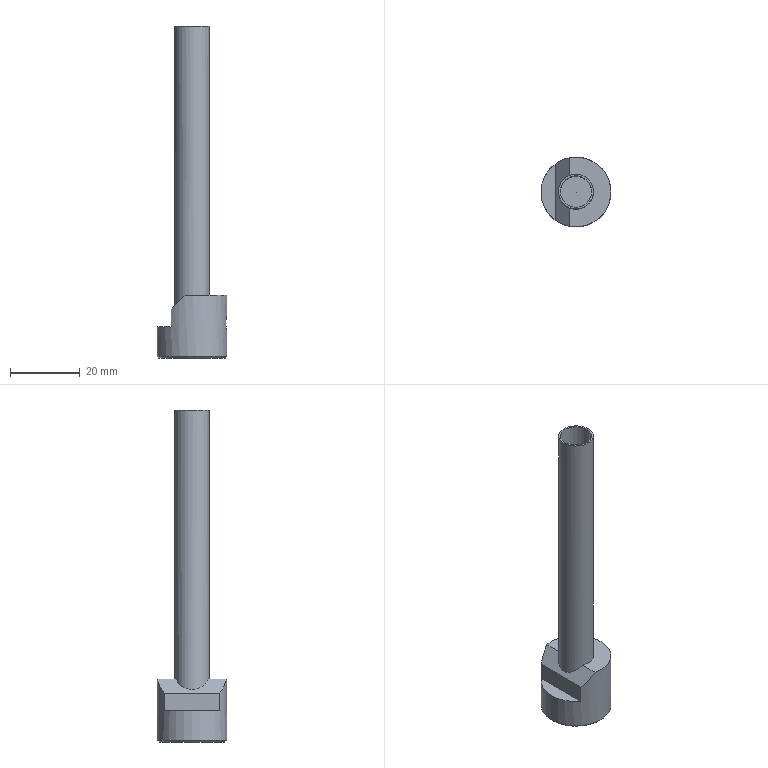Part | STEP file | SL2-MOLD_id178_xmt_txt | 1 solid | 15 faces | box 20 x 20 x 95 mm | volume 5358 mm3 | plane 7 | cylinder 5 | cone 3 | commonest cylinder face diameters 3.3 x1 5 x1 9 x1 10 x1 20 x1
STEP:
#1=CARTESIAN_POINT('',(43.,-50.,-35.));
#2=VERTEX_POINT('',#1);
#3=CARTESIAN_POINT('',(43.,-50.,-40.));
#4=VERTEX_POINT('',#3);
#5=CARTESIAN_POINT('',(43.,-50.,-37.5));
#6=DIRECTION('',(0.,0.,-1.));
#7=VECTOR('',#6,1.);
#8=LINE('',#5,#7);
#9=EDGE_CURVE('',#2,#4,#8,.T.);
#10=ORIENTED_EDGE('',*,*,#9,.F.);
#11=CARTESIAN_POINT('',(43.,-34.,-35.));
#12=VERTEX_POINT('',#11);
#13=CARTESIAN_POINT('',(43.,-42.,-35.));
#14=DIRECTION('',(0.,1.,0.));
#15=VECTOR('',#14,1.);
#16=LINE('',#13,#15);
#17=EDGE_CURVE('',#2,#12,#16,.T.);
#18=ORIENTED_EDGE('',*,*,#17,.T.);
#19=CARTESIAN_POINT('',(43.,-34.,-40.));
#20=VERTEX_POINT('',#19);
#21=CARTESIAN_POINT('',(43.,-34.,-37.5));
#22=DIRECTION('',(0.,0.,1.));
#23=VECTOR('',#22,1.);
#24=LINE('',#21,#23);
#25=EDGE_CURVE('',#20,#12,#24,.T.);
#26=ORIENTED_EDGE('',*,*,#25,.F.);
#27=CARTESIAN_POINT('',(43.,-42.,-40.));
#28=DIRECTION('',(0.,1.,0.));
#29=VECTOR('',#28,1.);
#30=LINE('',#27,#29);
#31=EDGE_CURVE('',#4,#20,#30,.T.);
#32=ORIENTED_EDGE('',*,*,#31,.F.);
#33=EDGE_LOOP('',(#10,#18,#26,#32));
#34=FACE_OUTER_BOUND('',#33,.T.);
#35=CARTESIAN_POINT('',(43.,-42.,-46.));
#36=DIRECTION('',(-1.,0.,0.));
#37=DIRECTION('',(0.,0.,1.));
#38=AXIS2_PLACEMENT_3D('',#35,#36,#37);
#39=PLANE('',#38);
#40=ADVANCED_FACE('',(#34),#39,.T.);
#41=CARTESIAN_POINT('',(47.,-51.798,-31.));
#42=VERTEX_POINT('',#41);
#43=CARTESIAN_POINT('',(47.,-32.202,-31.));
#44=VERTEX_POINT('',#43);
#45=CARTESIAN_POINT('',(49.,-42.,-31.));
#46=DIRECTION('',(0.,0.,1.));
#47=DIRECTION('',(-1.,0.,0.));
#48=AXIS2_PLACEMENT_3D('',#45,#46,#47);
#49=CIRCLE('',#48,10.);
#50=EDGE_CURVE('',#42,#44,#49,.T.);
#51=ORIENTED_EDGE('',*,*,#50,.T.);
#52=CARTESIAN_POINT('',(47.,-37.417,-31.));
#53=VERTEX_POINT('',#52);
#54=CARTESIAN_POINT('',(47.,-42.,-31.));
#55=DIRECTION('',(0.,-1.,0.));
#56=VECTOR('',#55,1.);
#57=LINE('',#54,#56);
#58=EDGE_CURVE('',#44,#53,#57,.T.);
#59=ORIENTED_EDGE('',*,*,#58,.T.);
#60=CARTESIAN_POINT('',(47.,-46.583,-31.));
#61=VERTEX_POINT('',#60);
#62=CARTESIAN_POINT('',(49.,-42.,-31.));
#63=DIRECTION('',(0.,0.,-1.));
#64=DIRECTION('',(-1.,0.,0.));
#65=AXIS2_PLACEMENT_3D('',#62,#63,#64);
#66=CIRCLE('',#65,5.);
#67=EDGE_CURVE('',#53,#61,#66,.T.);
#68=ORIENTED_EDGE('',*,*,#67,.T.);
#69=CARTESIAN_POINT('',(47.,-42.,-31.));
#70=DIRECTION('',(0.,-1.,0.));
#71=VECTOR('',#70,1.);
#72=LINE('',#69,#71);
#73=EDGE_CURVE('',#61,#42,#72,.T.);
#74=ORIENTED_EDGE('',*,*,#73,.T.);
#75=EDGE_LOOP('',(#51,#59,#68,#74));
#76=FACE_OUTER_BOUND('',#75,.T.);
#77=CARTESIAN_POINT('',(49.,-42.,-31.));
#78=DIRECTION('',(0.,0.,-1.));
#79=DIRECTION('',(-1.,0.,0.));
#80=AXIS2_PLACEMENT_3D('',#77,#78,#79);
#81=PLANE('',#80);
#82=ADVANCED_FACE('',(#76),#81,.F.);
#83=CARTESIAN_POINT('',(39.,-42.,-48.5));
#84=VERTEX_POINT('',#83);
#85=CARTESIAN_POINT('',(49.,-42.,-48.5));
#86=DIRECTION('',(0.,0.,1.));
#87=DIRECTION('',(-1.,0.,0.));
#88=AXIS2_PLACEMENT_3D('',#85,#86,#87);
#89=CIRCLE('',#88,10.);
#90=EDGE_CURVE('',#84,#84,#89,.T.);
#91=ORIENTED_EDGE('',*,*,#90,.T.);
#92=EDGE_LOOP('',(#91));
#93=FACE_BOUND('',#92,.T.);
#94=CARTESIAN_POINT('',(58.927,-40.795,-36.81));
#95=VERTEX_POINT('',#94);
#96=CARTESIAN_POINT('',(58.927,-40.795,-36.81));
#97=CARTESIAN_POINT('',(58.956,-41.034,-36.678));
#98=CARTESIAN_POINT('',(58.979,-41.3,-36.584));
#99=CARTESIAN_POINT('',(58.991,-41.57,-36.537));
#100=CARTESIAN_POINT('',(59.002,-41.841,-36.49));
#101=CARTESIAN_POINT('',(59.003,-42.124,-36.488));
#102=CARTESIAN_POINT('',(58.992,-42.395,-36.531));
#103=CARTESIAN_POINT('',(58.982,-42.663,-36.574));
#104=CARTESIAN_POINT('',(58.96,-42.927,-36.663));
#105=CARTESIAN_POINT('',(58.932,-43.166,-36.789));
#106=CARTESIAN_POINT('',(58.903,-43.409,-36.917));
#107=CARTESIAN_POINT('',(58.868,-43.632,-37.087));
#108=CARTESIAN_POINT('',(58.833,-43.82,-37.286));
#109=CARTESIAN_POINT('',(58.797,-44.012,-37.49));
#110=CARTESIAN_POINT('',(58.762,-44.172,-37.731));
#111=CARTESIAN_POINT('',(58.735,-44.286,-37.989));
#112=CARTESIAN_POINT('',(58.708,-44.4,-38.246));
#113=CARTESIAN_POINT('',(58.69,-44.471,-38.527));
#114=CARTESIAN_POINT('',(58.684,-44.493,-38.809));
#115=CARTESIAN_POINT('',(58.679,-44.514,-39.082));
#116=CARTESIAN_POINT('',(58.686,-44.489,-39.363));
#117=CARTESIAN_POINT('',(58.703,-44.42,-39.628));
#118=CARTESIAN_POINT('',(58.72,-44.352,-39.891));
#119=CARTESIAN_POINT('',(58.747,-44.239,-40.145));
#120=CARTESIAN_POINT('',(58.779,-44.091,-40.37));
#121=CARTESIAN_POINT('',(58.811,-43.94,-40.601));
#122=CARTESIAN_POINT('',(58.849,-43.747,-40.809));
#123=CARTESIAN_POINT('',(58.882,-43.529,-40.978));
#124=CARTESIAN_POINT('',(58.917,-43.306,-41.151));
#125=CARTESIAN_POINT('',(58.948,-43.049,-41.287));
#126=CARTESIAN_POINT('',(58.97,-42.78,-41.375));
#127=CARTESIAN_POINT('',(58.99,-42.515,-41.462));
#128=CARTESIAN_POINT('',(59.001,-42.229,-41.505));
#129=CARTESIAN_POINT('',(59.,-41.949,-41.499));
#130=CARTESIAN_POINT('',(58.998,-41.677,-41.494));
#131=CARTESIAN_POINT('',(58.985,-41.401,-41.442));
#132=CARTESIAN_POINT('',(58.963,-41.145,-41.349));
#133=CARTESIAN_POINT('',(58.941,-40.889,-41.256));
#134=CARTESIAN_POINT('',(58.91,-40.647,-41.119));
#135=CARTESIAN_POINT('',(58.877,-40.435,-40.95));
#136=CARTESIAN_POINT('',(58.842,-40.218,-40.776));
#137=CARTESIAN_POINT('',(58.805,-40.028,-40.562));
#138=CARTESIAN_POINT('',(58.773,-39.881,-40.326));
#139=CARTESIAN_POINT('',(58.74,-39.731,-40.087));
#140=CARTESIAN_POINT('',(58.713,-39.621,-39.818));
#141=CARTESIAN_POINT('',(58.698,-39.559,-39.541));
#142=CARTESIAN_POINT('',(58.682,-39.499,-39.27));
#143=CARTESIAN_POINT('',(58.679,-39.485,-38.984));
#144=CARTESIAN_POINT('',(58.687,-39.517,-38.708));
#145=CARTESIAN_POINT('',(58.695,-39.549,-38.439));
#146=CARTESIAN_POINT('',(58.715,-39.626,-38.171));
#147=CARTESIAN_POINT('',(58.742,-39.742,-37.927));
#148=CARTESIAN_POINT('',(58.769,-39.859,-37.68));
#149=CARTESIAN_POINT('',(58.804,-40.019,-37.451));
#150=CARTESIAN_POINT('',(58.838,-40.209,-37.255));
#151=CARTESIAN_POINT('',(58.869,-40.38,-37.08));
#152=CARTESIAN_POINT('',(58.901,-40.58,-36.928));
#153=CARTESIAN_POINT('',(58.927,-40.795,-36.81));
#154=B_SPLINE_CURVE_WITH_KNOTS('',3,(#96,#97,#98,#99,#100,#101,#102,#103,#104,#105,#106,#107,#108,#109,#110,#111,#112,#113,#114,#115,#116,#117,#118,#119,#120,#121,#122,#123,#124,#125,#126,#127,#128,#129,#130,#131,#132,#133,#134,#135,#136,#137,#138,#139,#140,#141,#142,#143,#144,#145,#146,#147,#148,#149,#150,#151,#152,#153),.UNSPECIFIED.,.T.,.F.,(1,3,3,3,3,3,3,3,3,3,3,3,3,3,3,3,3,3,3,3,3,1),(-0.04706,0.,0.05251,0.1051,0.157,0.2097,0.2638,0.3178,0.3703,0.4222,0.4753,0.5296,0.5832,0.6354,0.6876,0.7411,0.7954,0.8486,0.9005,0.9529,1.,1.053),.UNSPECIFIED.);
#155=EDGE_CURVE('',#95,#95,#154,.T.);
#156=ORIENTED_EDGE('',*,*,#155,.F.);
#157=EDGE_LOOP('',(#156));
#158=FACE_BOUND('',#157,.T.);
#159=ORIENTED_EDGE('',*,*,#25,.T.);
#160=CARTESIAN_POINT('',(49.,-42.,-29.));
#161=DIRECTION('',(0.7071,0.,-0.7071));
#162=DIRECTION('',(0.7071,0.,0.7071));
#163=AXIS2_PLACEMENT_3D('',#160,#161,#162);
#164=ELLIPSE('',#163,14.142,10.);
#165=EDGE_CURVE('',#12,#44,#164,.T.);
#166=ORIENTED_EDGE('',*,*,#165,.T.);
#167=ORIENTED_EDGE('',*,*,#50,.F.);
#168=CARTESIAN_POINT('',(49.,-42.,-29.));
#169=DIRECTION('',(0.7071,0.,-0.7071));
#170=DIRECTION('',(0.7071,0.,0.7071));
#171=AXIS2_PLACEMENT_3D('',#168,#169,#170);
#172=ELLIPSE('',#171,14.142,10.);
#173=EDGE_CURVE('',#42,#2,#172,.T.);
#174=ORIENTED_EDGE('',*,*,#173,.T.);
#175=ORIENTED_EDGE('',*,*,#9,.T.);
#176=CARTESIAN_POINT('',(49.,-42.,-40.));
#177=DIRECTION('',(0.,0.,1.));
#178=DIRECTION('',(1.,0.,0.));
#179=AXIS2_PLACEMENT_3D('',#176,#177,#178);
#180=CIRCLE('',#179,10.);
#181=EDGE_CURVE('',#20,#4,#180,.T.);
#182=ORIENTED_EDGE('',*,*,#181,.F.);
#183=EDGE_LOOP('',(#159,#166,#167,#174,#175,#182));
#184=FACE_BOUND('',#183,.T.);
#185=CARTESIAN_POINT('',(49.,-42.,-46.));
#186=DIRECTION('',(0.,0.,1.));
#187=DIRECTION('',(-1.,0.,0.));
#188=AXIS2_PLACEMENT_3D('',#185,#186,#187);
#189=CYLINDRICAL_SURFACE('',#188,10.);
#190=ADVANCED_FACE('',(#93,#158,#184),#189,.T.);
#191=CARTESIAN_POINT('',(39.5,-42.,-49.));
#192=VERTEX_POINT('',#191);
#193=CARTESIAN_POINT('',(49.,-42.,-49.));
#194=DIRECTION('',(0.,0.,-1.));
#195=DIRECTION('',(-1.,0.,0.));
#196=AXIS2_PLACEMENT_3D('',#193,#194,#195);
#197=CIRCLE('',#196,9.5);
#198=EDGE_CURVE('',#192,#192,#197,.T.);
#199=ORIENTED_EDGE('',*,*,#198,.T.);
#200=EDGE_LOOP('',(#199));
#201=FACE_BOUND('',#200,.T.);
#202=CARTESIAN_POINT('',(47.,-42.,-49.));
#203=VERTEX_POINT('',#202);
#204=CARTESIAN_POINT('',(49.,-42.,-49.));
#205=DIRECTION('',(0.,0.,1.));
#206=DIRECTION('',(-1.,0.,0.));
#207=AXIS2_PLACEMENT_3D('',#204,#205,#206);
#208=CIRCLE('',#207,2.);
#209=EDGE_CURVE('',#203,#203,#208,.T.);
#210=ORIENTED_EDGE('',*,*,#209,.T.);
#211=EDGE_LOOP('',(#210));
#212=FACE_BOUND('',#211,.T.);
#213=CARTESIAN_POINT('',(49.,-42.,-49.));
#214=DIRECTION('',(0.,0.,-1.));
#215=DIRECTION('',(-1.,0.,0.));
#216=AXIS2_PLACEMENT_3D('',#213,#214,#215);
#217=PLANE('',#216);
#218=ADVANCED_FACE('',(#201,#212),#217,.T.);
#219=ORIENTED_EDGE('',*,*,#181,.T.);
#220=ORIENTED_EDGE('',*,*,#31,.T.);
#221=EDGE_LOOP('',(#219,#220));
#222=FACE_OUTER_BOUND('',#221,.T.);
#223=CARTESIAN_POINT('',(43.,-42.,-40.));
#224=DIRECTION('',(0.,0.,1.));
#225=DIRECTION('',(1.,0.,0.));
#226=AXIS2_PLACEMENT_3D('',#223,#224,#225);
#227=PLANE('',#226);
#228=ADVANCED_FACE('',(#222),#227,.T.);
#229=CARTESIAN_POINT('',(52.742,-39.5,-39.));
#230=VERTEX_POINT('',#229);
#231=CARTESIAN_POINT('',(52.742,-44.5,-39.));
#232=VERTEX_POINT('',#231);
#233=CARTESIAN_POINT('',(52.742,-39.5,-39.));
#234=CARTESIAN_POINT('',(52.742,-39.5,-38.763));
#235=CARTESIAN_POINT('',(52.765,-39.535,-38.524));
#236=CARTESIAN_POINT('',(52.807,-39.6,-38.3));
#237=CARTESIAN_POINT('',(52.848,-39.666,-38.073));
#238=CARTESIAN_POINT('',(52.908,-39.764,-37.857));
#239=CARTESIAN_POINT('',(52.973,-39.888,-37.663));
#240=CARTESIAN_POINT('',(53.049,-40.029,-37.439));
#241=CARTESIAN_POINT('',(53.133,-40.208,-37.237));
#242=CARTESIAN_POINT('',(53.211,-40.412,-37.069));
#243=CARTESIAN_POINT('',(53.296,-40.638,-36.884));
#244=CARTESIAN_POINT('',(53.374,-40.903,-36.734));
#245=CARTESIAN_POINT('',(53.426,-41.186,-36.636));
#246=CARTESIAN_POINT('',(53.473,-41.443,-36.548));
#247=CARTESIAN_POINT('',(53.5,-41.724,-36.5));
#248=CARTESIAN_POINT('',(53.5,-42.,-36.5));
#249=CARTESIAN_POINT('',(53.5,-42.258,-36.5));
#250=CARTESIAN_POINT('',(53.477,-42.52,-36.541));
#251=CARTESIAN_POINT('',(53.435,-42.763,-36.619));
#252=CARTESIAN_POINT('',(53.393,-43.005,-36.697));
#253=CARTESIAN_POINT('',(53.333,-43.234,-36.812));
#254=CARTESIAN_POINT('',(53.264,-43.437,-36.954));
#255=CARTESIAN_POINT('',(53.191,-43.655,-37.107));
#256=CARTESIAN_POINT('',(53.107,-43.848,-37.295));
#257=CARTESIAN_POINT('',(53.028,-44.005,-37.507));
#258=CARTESIAN_POINT('',(52.942,-44.179,-37.74));
#259=CARTESIAN_POINT('',(52.86,-44.315,-38.01));
#260=CARTESIAN_POINT('',(52.807,-44.399,-38.296));
#261=CARTESIAN_POINT('',(52.766,-44.465,-38.521));
#262=CARTESIAN_POINT('',(52.742,-44.5,-38.762));
#263=CARTESIAN_POINT('',(52.742,-44.5,-39.));
#264=B_SPLINE_CURVE_WITH_KNOTS('',3,(#233,#234,#235,#236,#237,#238,#239,#240,#241,#242,#243,#244,#245,#246,#247,#248,#249,#250,#251,#252,#253,#254,#255,#256,#257,#258,#259,#260,#261,#262,#263),.UNSPECIFIED.,.F.,.F.,(4,3,3,3,3,3,3,3,3,3,4),(0.,0.08871,0.1782,0.2814,0.3957,0.4995,0.5966,0.6932,0.7966,0.9107,1.),.UNSPECIFIED.);
#265=EDGE_CURVE('',#230,#232,#264,.T.);
#266=ORIENTED_EDGE('',*,*,#265,.T.);
#267=CARTESIAN_POINT('',(52.742,-44.5,-39.));
#268=CARTESIAN_POINT('',(52.742,-44.5,-39.237));
#269=CARTESIAN_POINT('',(52.765,-44.465,-39.476));
#270=CARTESIAN_POINT('',(52.807,-44.4,-39.7));
#271=CARTESIAN_POINT('',(52.848,-44.334,-39.927));
#272=CARTESIAN_POINT('',(52.908,-44.236,-40.143));
#273=CARTESIAN_POINT('',(52.973,-44.112,-40.337));
#274=CARTESIAN_POINT('',(53.049,-43.971,-40.561));
#275=CARTESIAN_POINT('',(53.133,-43.792,-40.763));
#276=CARTESIAN_POINT('',(53.211,-43.588,-40.931));
#277=CARTESIAN_POINT('',(53.296,-43.362,-41.116));
#278=CARTESIAN_POINT('',(53.374,-43.097,-41.266));
#279=CARTESIAN_POINT('',(53.426,-42.814,-41.364));
#280=CARTESIAN_POINT('',(53.473,-42.557,-41.452));
#281=CARTESIAN_POINT('',(53.5,-42.276,-41.5));
#282=CARTESIAN_POINT('',(53.5,-42.,-41.5));
#283=CARTESIAN_POINT('',(53.5,-41.742,-41.5));
#284=CARTESIAN_POINT('',(53.477,-41.48,-41.459));
#285=CARTESIAN_POINT('',(53.435,-41.237,-41.381));
#286=CARTESIAN_POINT('',(53.393,-40.995,-41.303));
#287=CARTESIAN_POINT('',(53.333,-40.766,-41.188));
#288=CARTESIAN_POINT('',(53.264,-40.563,-41.046));
#289=CARTESIAN_POINT('',(53.191,-40.345,-40.893));
#290=CARTESIAN_POINT('',(53.107,-40.152,-40.705));
#291=CARTESIAN_POINT('',(53.028,-39.995,-40.493));
#292=CARTESIAN_POINT('',(52.942,-39.821,-40.26));
#293=CARTESIAN_POINT('',(52.86,-39.685,-39.99));
#294=CARTESIAN_POINT('',(52.807,-39.601,-39.704));
#295=CARTESIAN_POINT('',(52.766,-39.535,-39.479));
#296=CARTESIAN_POINT('',(52.742,-39.5,-39.238));
#297=CARTESIAN_POINT('',(52.742,-39.5,-39.));
#298=B_SPLINE_CURVE_WITH_KNOTS('',3,(#267,#268,#269,#270,#271,#272,#273,#274,#275,#276,#277,#278,#279,#280,#281,#282,#283,#284,#285,#286,#287,#288,#289,#290,#291,#292,#293,#294,#295,#296,#297),.UNSPECIFIED.,.F.,.F.,(4,3,3,3,3,3,3,3,3,3,4),(0.,0.08871,0.1782,0.2814,0.3957,0.4995,0.5966,0.6932,0.7966,0.9107,1.),.UNSPECIFIED.);
#299=EDGE_CURVE('',#232,#230,#298,.T.);
#300=ORIENTED_EDGE('',*,*,#299,.T.);
#301=EDGE_LOOP('',(#266,#300));
#302=FACE_BOUND('',#301,.T.);
#303=CARTESIAN_POINT('',(44.5,-42.,-43.));
#304=VERTEX_POINT('',#303);
#305=CARTESIAN_POINT('',(49.,-42.,-43.));
#306=DIRECTION('',(0.,0.,1.));
#307=DIRECTION('',(-1.,0.,0.));
#308=AXIS2_PLACEMENT_3D('',#305,#306,#307);
#309=CIRCLE('',#308,4.5);
#310=EDGE_CURVE('',#304,#304,#309,.T.);
#311=ORIENTED_EDGE('',*,*,#310,.F.);
#312=EDGE_LOOP('',(#311));
#313=FACE_BOUND('',#312,.T.);
#314=CARTESIAN_POINT('',(53.5,-42.,46.));
#315=VERTEX_POINT('',#314);
#316=CARTESIAN_POINT('',(49.,-42.,46.));
#317=DIRECTION('',(0.,0.,-1.));
#318=DIRECTION('',(1.,0.,0.));
#319=AXIS2_PLACEMENT_3D('',#316,#317,#318);
#320=CIRCLE('',#319,4.5);
#321=EDGE_CURVE('',#315,#315,#320,.T.);
#322=ORIENTED_EDGE('',*,*,#321,.F.);
#323=EDGE_LOOP('',(#322));
#324=FACE_BOUND('',#323,.T.);
#325=CARTESIAN_POINT('',(49.,-42.,-34.));
#326=DIRECTION('',(0.,0.,-1.));
#327=DIRECTION('',(-1.,0.,0.));
#328=AXIS2_PLACEMENT_3D('',#325,#326,#327);
#329=CYLINDRICAL_SURFACE('',#328,4.5);
#330=ADVANCED_FACE('',(#302,#313,#324),#329,.F.);
#331=ORIENTED_EDGE('',*,*,#310,.T.);
#332=EDGE_LOOP('',(#331));
#333=FACE_OUTER_BOUND('',#332,.T.);
#334=CARTESIAN_POINT('',(49.,-42.,-43.));
#335=DIRECTION('',(0.,0.,-1.));
#336=DIRECTION('',(-1.,0.,0.));
#337=AXIS2_PLACEMENT_3D('',#334,#335,#336);
#338=PLANE('',#337);
#339=ADVANCED_FACE('',(#333),#338,.F.);
#340=CARTESIAN_POINT('',(50.65,-42.,-44.));
#341=VERTEX_POINT('',#340);
#342=CARTESIAN_POINT('',(49.,-42.,-44.));
#343=DIRECTION('',(0.,0.,-1.));
#344=DIRECTION('',(1.,0.,0.));
#345=AXIS2_PLACEMENT_3D('',#342,#343,#344);
#346=CIRCLE('',#345,1.65);
#347=EDGE_CURVE('',#341,#341,#346,.T.);
#348=ORIENTED_EDGE('',*,*,#347,.T.);
#349=EDGE_LOOP('',(#348));
#350=FACE_BOUND('',#349,.T.);
#351=CARTESIAN_POINT('',(49.,-42.,-43.009));
#352=VERTEX_POINT('',#351);
#353=VERTEX_LOOP('',#352);
#354=FACE_BOUND('',#353,.T.);
#355=CARTESIAN_POINT('',(49.,-42.,-44.));
#356=DIRECTION('',(0.,0.,-1.));
#357=DIRECTION('',(-1.,0.,0.));
#358=AXIS2_PLACEMENT_3D('',#355,#356,#357);
#359=CONICAL_SURFACE('',#358,1.65,59.);
#360=ADVANCED_FACE('',(#350,#354),#359,.F.);
#361=CARTESIAN_POINT('',(47.35,-42.,-48.65));
#362=VERTEX_POINT('',#361);
#363=CARTESIAN_POINT('',(49.,-42.,-48.65));
#364=DIRECTION('',(0.,0.,-1.));
#365=DIRECTION('',(-1.,0.,0.));
#366=AXIS2_PLACEMENT_3D('',#363,#364,#365);
#367=CIRCLE('',#366,1.65);
#368=EDGE_CURVE('',#362,#362,#367,.T.);
#369=ORIENTED_EDGE('',*,*,#368,.T.);
#370=EDGE_LOOP('',(#369));
#371=FACE_BOUND('',#370,.T.);
#372=ORIENTED_EDGE('',*,*,#347,.F.);
#373=EDGE_LOOP('',(#372));
#374=FACE_BOUND('',#373,.T.);
#375=CARTESIAN_POINT('',(49.,-42.,-49.));
#376=DIRECTION('',(0.,0.,1.));
#377=DIRECTION('',(1.,0.,0.));
#378=AXIS2_PLACEMENT_3D('',#375,#376,#377);
#379=CYLINDRICAL_SURFACE('',#378,1.65);
#380=ADVANCED_FACE('',(#371,#374),#379,.F.);
#381=ORIENTED_EDGE('',*,*,#368,.F.);
#382=EDGE_LOOP('',(#381));
#383=FACE_BOUND('',#382,.T.);
#384=ORIENTED_EDGE('',*,*,#209,.F.);
#385=EDGE_LOOP('',(#384));
#386=FACE_BOUND('',#385,.T.);
#387=CARTESIAN_POINT('',(49.,-42.,-49.));
#388=DIRECTION('',(0.,0.,-1.));
#389=DIRECTION('',(-1.,0.,0.));
#390=AXIS2_PLACEMENT_3D('',#387,#388,#389);
#391=CONICAL_SURFACE('',#390,2.,45.);
#392=ADVANCED_FACE('',(#383,#386),#391,.F.);
#393=ORIENTED_EDGE('',*,*,#67,.F.);
#394=CARTESIAN_POINT('',(49.,-42.,-29.));
#395=DIRECTION('',(-0.7071,0.,0.7071));
#396=DIRECTION('',(0.7071,0.,0.7071));
#397=AXIS2_PLACEMENT_3D('',#394,#395,#396);
#398=ELLIPSE('',#397,7.071,5.);
#399=EDGE_CURVE('',#53,#61,#398,.T.);
#400=ORIENTED_EDGE('',*,*,#399,.T.);
#401=EDGE_LOOP('',(#393,#400));
#402=FACE_BOUND('',#401,.T.);
#403=CARTESIAN_POINT('',(54.,-42.,46.));
#404=VERTEX_POINT('',#403);
#405=CARTESIAN_POINT('',(49.,-42.,46.));
#406=DIRECTION('',(0.,0.,-1.));
#407=DIRECTION('',(1.,0.,0.));
#408=AXIS2_PLACEMENT_3D('',#405,#406,#407);
#409=CIRCLE('',#408,5.);
#410=EDGE_CURVE('',#404,#404,#409,.T.);
#411=ORIENTED_EDGE('',*,*,#410,.T.);
#412=EDGE_LOOP('',(#411));
#413=FACE_BOUND('',#412,.T.);
#414=CARTESIAN_POINT('',(49.,-42.,-46.));
#415=DIRECTION('',(0.,0.,1.));
#416=DIRECTION('',(-1.,0.,0.));
#417=AXIS2_PLACEMENT_3D('',#414,#415,#416);
#418=CYLINDRICAL_SURFACE('',#417,5.);
#419=ADVANCED_FACE('',(#402,#413),#418,.T.);
#420=ORIENTED_EDGE('',*,*,#321,.T.);
#421=EDGE_LOOP('',(#420));
#422=FACE_BOUND('',#421,.T.);
#423=ORIENTED_EDGE('',*,*,#410,.F.);
#424=EDGE_LOOP('',(#423));
#425=FACE_BOUND('',#424,.T.);
#426=CARTESIAN_POINT('',(49.,-42.,46.));
#427=DIRECTION('',(0.,0.,1.));
#428=DIRECTION('',(1.,0.,0.));
#429=AXIS2_PLACEMENT_3D('',#426,#427,#428);
#430=PLANE('',#429);
#431=ADVANCED_FACE('',(#422,#425),#430,.T.);
#432=ORIENTED_EDGE('',*,*,#155,.T.);
#433=EDGE_LOOP('',(#432));
#434=FACE_BOUND('',#433,.T.);
#435=ORIENTED_EDGE('',*,*,#299,.F.);
#436=ORIENTED_EDGE('',*,*,#265,.F.);
#437=EDGE_LOOP('',(#435,#436));
#438=FACE_BOUND('',#437,.T.);
#439=CARTESIAN_POINT('',(49.,-42.,-39.));
#440=DIRECTION('',(1.,0.,0.));
#441=DIRECTION('',(0.,0.,-1.));
#442=AXIS2_PLACEMENT_3D('',#439,#440,#441);
#443=CYLINDRICAL_SURFACE('',#442,2.5);
#444=ADVANCED_FACE('',(#434,#438),#443,.F.);
#445=ORIENTED_EDGE('',*,*,#399,.F.);
#446=ORIENTED_EDGE('',*,*,#58,.F.);
#447=ORIENTED_EDGE('',*,*,#165,.F.);
#448=ORIENTED_EDGE('',*,*,#17,.F.);
#449=ORIENTED_EDGE('',*,*,#173,.F.);
#450=ORIENTED_EDGE('',*,*,#73,.F.);
#451=EDGE_LOOP('',(#445,#446,#447,#448,#449,#450));
#452=FACE_OUTER_BOUND('',#451,.T.);
#453=CARTESIAN_POINT('',(43.,-42.,-35.));
#454=DIRECTION('',(-0.7071,0.,0.7071));
#455=DIRECTION('',(0.7071,0.,0.7071));
#456=AXIS2_PLACEMENT_3D('',#453,#454,#455);
#457=PLANE('',#456);
#458=ADVANCED_FACE('',(#452),#457,.T.);
#459=ORIENTED_EDGE('',*,*,#198,.F.);
#460=EDGE_LOOP('',(#459));
#461=FACE_BOUND('',#460,.T.);
#462=ORIENTED_EDGE('',*,*,#90,.F.);
#463=EDGE_LOOP('',(#462));
#464=FACE_BOUND('',#463,.T.);
#465=CARTESIAN_POINT('',(49.,-42.,-48.5));
#466=DIRECTION('',(0.,0.,1.));
#467=DIRECTION('',(1.,0.,0.));
#468=AXIS2_PLACEMENT_3D('',#465,#466,#467);
#469=CONICAL_SURFACE('',#468,10.,45.);
#470=ADVANCED_FACE('',(#461,#464),#469,.T.);
#471=CLOSED_SHELL('',(#40,#82,#190,#218,#228,#330,#339,#360,#380,#392,#419,#431,#444,#458,#470));
#472=MANIFOLD_SOLID_BREP('',#471);
#473=(LENGTH_UNIT()NAMED_UNIT(*)SI_UNIT(.MILLI.,.METRE.));
#474=UNCERTAINTY_MEASURE_WITH_UNIT(LENGTH_MEASURE(0.0508),#473,'','');
#475=(NAMED_UNIT(*)PLANE_ANGLE_UNIT()SI_UNIT($,.RADIAN.));
#476=PLANE_ANGLE_MEASURE_WITH_UNIT(PLANE_ANGLE_MEASURE(0.01745),#475);
#477=DIMENSIONAL_EXPONENTS(0.,0.,0.,0.,0.,0.,0.);
#478=(CONVERSION_BASED_UNIT('DEGREE',#476)NAMED_UNIT(#477)PLANE_ANGLE_UNIT());
#479=(NAMED_UNIT(*)SI_UNIT($,.STERADIAN.)SOLID_ANGLE_UNIT());
#480=(GEOMETRIC_REPRESENTATION_CONTEXT(3)GLOBAL_UNCERTAINTY_ASSIGNED_CONTEXT((#474))GLOBAL_UNIT_ASSIGNED_CONTEXT((#473,#478,#479))REPRESENTATION_CONTEXT('',''));
#481=ADVANCED_BREP_SHAPE_REPRESENTATION('',(#472),#480);